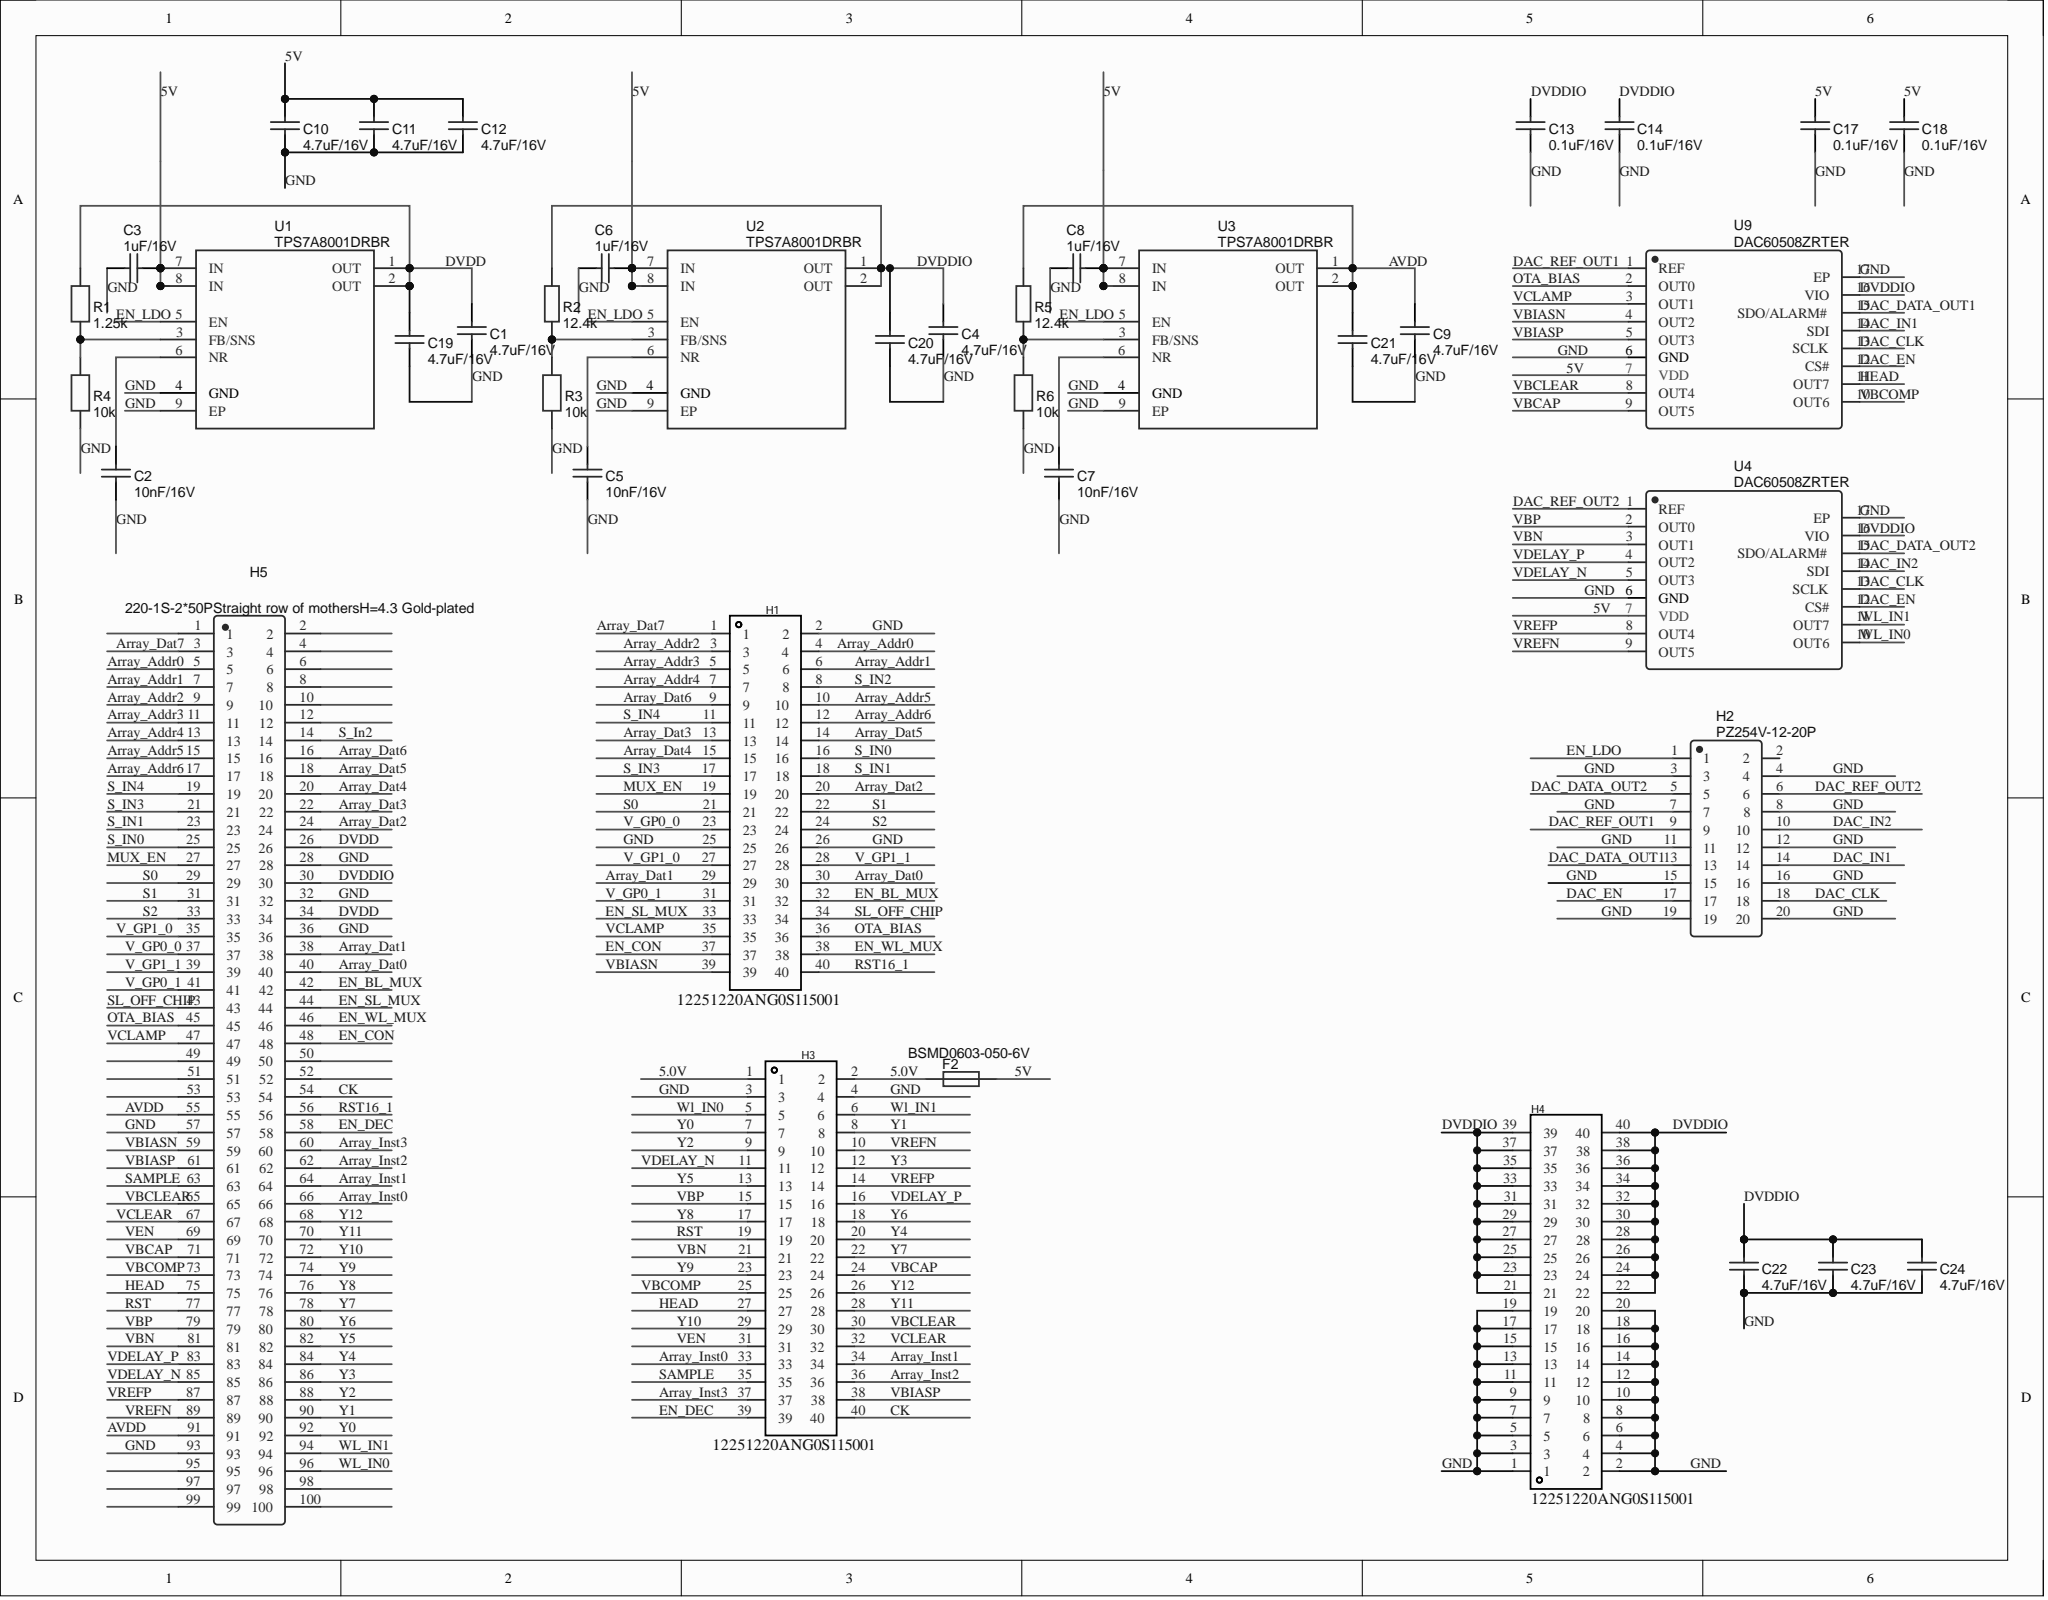Circuit board | Altium Designer | 39 parts | 94 nets
Bill of materials:
Comment,Description,Designator,Footprint,LibRef,Quantity
"4.7uF/16V","","C1, C4, C9, C10, C11, C12, C19, C20, C21, C22, C23, C24","C0603","4.7uF","12"
"10nF/16V","","C2, C5, C7","C0603","10nF","3"
"1uF/16V","","C3, C6, C8","C0603","1uF","3"
"0.1uF/16V","","C13, C14, C17, C18","C0603","10nF","4"
"BSMD0603-050-6V","","F2","F0603","BSMD0603-050-6V","1"
"12251220ANG0S115001","","H1, H3, H4","HDR-TH_40P-P2.54-V-M-R2-C20-S2.54","12251220ANG0S115001","3"
"PZ254V-12-20P","","H2","HDR-TH_20P-P2.54-V-M-R2-C10-S2.54","PZ254V-12-20P","1"
"220-1S-2*50PStraight row of mothersH=4.3 Gold-plated","","H5","IC51-1004-809-23","220-1S-2*50PStraight row of mothersH=4.3 Gold-plated","1"
"1.25k","","R1","R0805","","1"
"12.4k","","R2, R5","R0805","","2"
"10k","","R3, R4, R6","R0805","","3"
"TPS7A8001DRBR","","U1, U2, U3","VSON-8_L3.0-W3.0-P0.65-TL-EP","TPS7A8001DRBR","3"
"DAC60508ZRTER","","U4, U9","WQFN-16_L3.0-W3.0-P0.50-BL-EP0.8","DAC60508ZRTER","2"
Netlist (Protel format):
[
C1
C0603
4.7uF/16V



]
[
C2
C0603
10nF/16V



]
[
C3
C0603
1uF/16V



]
[
C4
C0603
4.7uF/16V



]
[
C5
C0603
10nF/16V



]
[
C6
C0603
1uF/16V



]
[
C7
C0603
10nF/16V



]
[
C8
C0603
1uF/16V



]
[
C9
C0603
4.7uF/16V



]
[
C10
C0603
4.7uF/16V



]
[
C11
C0603
4.7uF/16V



]
[
C12
C0603
4.7uF/16V



]
[
C13
C0603
0.1uF/16V



]
[
C14
C0603
0.1uF/16V



]
[
C17
C0603
0.1uF/16V



]
[
C18
C0603
0.1uF/16V



]
[
C19
C0603
4.7uF/16V



]
[
C20
C0603
4.7uF/16V



]
[
C21
C0603
4.7uF/16V



]
[
C22
C0603
4.7uF/16V



]
[
C23
C0603
4.7uF/16V



]
[
C24
C0603
4.7uF/16V



]
[
F2
F0603
BSMD0603-050-6V



]
[
H1
HDR-TH_40P-P2.54-V-M-R2-C20-S2.54
12251220ANG0S115001



]
[
H2
HDR-TH_20P-P2.54-V-M-R2-C10-S2.54
PZ254V-12-20P



]
[
H3
HDR-TH_40P-P2.54-V-M-R2-C20-S2.54
12251220ANG0S115001



]
[
H4
HDR-TH_40P-P2.54-V-M-R2-C20-S2.54
12251220ANG0S115001



]
[
H5
IC51-1004-809-23
220-1S-2*50PStraight row of mothersH=4.3 Gold-plated



]
[
R1
R0805
1.25k



]
[
R2
R0805
12.4k



]
[
R3
R0805
10k



]
[
R4
R0805
10k



]
[
R5
R0805
12.4k



]
[
R6
R0805
10k



]
[
U1
VSON-8_L3.0-W3.0-P0.65-TL-EP
TPS7A8001DRBR



]
[
U2
VSON-8_L3.0-W3.0-P0.65-TL-EP
TPS7A8001DRBR



]
[
U3
VSON-8_L3.0-W3.0-P0.65-TL-EP
TPS7A8001DRBR



]
[
U4
WQFN-16_L3.0-W3.0-P0.50-BL-EP0.8
DAC60508ZRTER



]
[
U9
WQFN-16_L3.0-W3.0-P0.50-BL-EP0.8
DAC60508ZRTER



]
(
Y12
H3-26
H5-68
)
(
Y11
H3-28
H5-70
)
(
Y10
H3-29
H5-72
)
(
Y9
H3-23
H5-74
)
(
Y8
H3-17
H5-76
)
(
Y7
H3-22
H5-78
)
(
Y6
H3-18
H5-80
)
(
Y5
H3-13
H5-82
)
(
Y4
H3-20
H5-84
)
(
Y3
H3-12
H5-86
)
(
Y2
H3-9
H5-88
)
(
Y1
H3-8
H5-90
)
(
Y0
H3-7
H5-92
)
(
Wl_IN1
H3-6
H5-94
U4-11
)
(
Wl_IN0
H3-5
H5-96
U4-10
)
(
VREFP
H3-14
H5-87
U4-8
)
(
VREFN
H3-10
H5-89
U4-9
)
(
VEN
H3-31
H5-69
)
(
VDELAY_P
H3-16
H5-83
U4-4
)
(
VDELAY_N
H3-11
H5-85
U4-5
)
(
VCLEAR
H3-32
H5-67
)
(
VCLAMP
H1-35
H5-47
U9-3
)
(
VBP
H3-15
H5-79
U4-2
)
(
VBN
H3-21
H5-81
U4-3
)
(
VBIASP
H3-38
H5-61
U9-5
)
(
VBIASN
H1-39
H5-59
U9-4
)
(
VBCOMP
H3-25
H5-73
U9-10
)
(
VBCLEAR
H3-30
H5-65
U9-8
)
(
VBCAP
H3-24
H5-71
U9-9
)
(
V_GP1_1
H1-28
H5-39
)
(
V_GP1_0
H1-27
H5-35
)
(
V_GP0_1
H1-31
H5-41
)
(
V_GP0_0
H1-23
H5-37
)
(
SL_OFF_CHIP
H1-34
H5-43
)
(
SAMPLE
H3-35
H5-63
)
(
S_IN4
H1-11
H5-19
)
(
S_IN3
H1-17
H5-21
)
(
S_In2
H1-8
H5-14
)
(
S_IN1
H1-18
H5-23
)
(
S_IN0
H1-16
H5-25
)
(
S2
H1-24
H5-33
)
(
S1
H1-22
H5-31
)
(
S0
H1-21
H5-29
)
(
RST16_1
H1-40
H5-56
)
(
RST
H3-19
H5-77
)
(
OTA_BIAS
H1-36
H5-45
U9-2
)
(
NetR5_2
R5-2
R6-2
U3-3
)
(
NetR2_2
R2-2
R3-2
U2-3
)
(
NetR1_2
R1-2
R4-2
U1-3
)
(
NetC7_2
C7-2
U3-6
)
(
NetC5_2
C5-2
U2-6
)
(
NetC2_2
C2-2
U1-6
)
(
MUX_EN
H1-19
H5-27
)
(
HEAD
H3-27
H5-75
U9-11
)
(
GND
C1-1
C2-1
C3-2
C4-1
C5-1
C6-2
C7-1
C8-2
C9-1
C10-1
C11-1
C12-1
C13-1
C14-1
C17-1
C18-1
C19-1
C20-1
C21-1
C22-1
C23-1
C24-1
H1-2
H1-25
H1-26
H2-3
H2-4
H2-7
H2-8
H2-11
H2-12
H2-15
H2-16
H2-19
H2-20
H3-3
H3-4
H4-1
H4-2
H4-3
H4-4
H4-5
H4-6
H4-7
H4-8
H4-9
H4-10
H4-11
H4-12
H4-13
H4-14
H4-15
H4-16
H4-17
H4-18
H4-19
H4-20
H5-28
H5-32
H5-36
H5-57
H5-93
R3-1
R4-1
R6-1
U1-4
U1-9
U2-4
U2-9
U3-4
U3-9
U4-6
U4-17
U9-6
U9-17
)
(
EN_WL_MUX
H1-38
H5-46
)
(
EN_SL_MUX
H1-33
H5-44
)
(
EN_LDO
H2-1
U1-5
U2-5
U3-5
)
(
EN_DEC
H3-39
H5-58
)
(
EN_CON
H1-37
H5-48
)
(
EN_BL_MUX
H1-32
H5-42
)
(
DVDDIO
C4-2
C13-2
C14-2
C20-2
C22-2
C23-2
C24-2
H4-21
H4-22
H4-23
H4-24
H4-25
H4-26
H4-27
H4-28
H4-29
H4-30
H4-31
H4-32
H4-33
H4-34
H4-35
H4-36
H4-37
H4-38
H4-39
H4-40
H5-30
R2-1
U2-1
U2-2
U4-16
U9-16
)
(
DVDD
C1-2
C19-2
H5-26
H5-34
R1-1
U1-1
U1-2
)
(
DAC_REF_OUT2
H2-6
U4-1
)
(
DAC_REF_OUT1
H2-9
U9-1
)
(
DAC_IN2
H2-10
U4-14
)
(
DAC_IN1
H2-14
U9-14
)
(
DAC_EN
H2-17
U4-12
U9-12
)
(
DAC_DATA_OUT2
H2-5
U4-15
)
(
DAC_DATA_OUT1
H2-13
U9-15
)
(
DAC_CLK
H2-18
U4-13
U9-13
)
(
CK
H3-40
H5-54
)
(
AVDD
C9-2
C21-2
H5-55
H5-91
R5-1
U3-1
U3-2
)
(
Array_Inst3
H3-37
H5-60
)
(
Array_Inst2
H3-36
H5-62
)
(
Array_Inst1
H3-34
H5-64
)
(
Array_Inst0
H3-33
H5-66
)
(
Array_Dat7
H1-1
H5-3
)
(
Array_Dat6
H1-9
H5-16
)
(
Array_Dat5
H1-14
H5-18
)
(
Array_Dat4
H1-15
H5-20
)
(
Array_Dat3
H1-13
H5-22
)
(
Array_Dat2
H1-20
H5-24
)
(
Array_Dat1
H1-29
H5-38
)
(
Array_Dat0
H1-30
H5-40
)
(
Array_Addr6
H1-12
H5-17
)
(
Array_Addr5
H1-10
H5-15
)
(
Array_Addr4
H1-7
H5-13
)
(
Array_Addr3
H1-5
H5-11
)
(
Array_Addr2
H1-3
H5-9
)
(
Array_Addr1
H1-6
H5-7
)
(
Array_Addr0
H1-4
H5-5
)
(
5V
C3-1
C6-1
C8-1
C10-2
C11-2
C12-2
C17-2
C18-2
F2-1
U1-7
U1-8
U2-7
U2-8
U3-7
U3-8
U4-7
U9-7
)
(
5.0V
F2-2
H3-1
H3-2
)